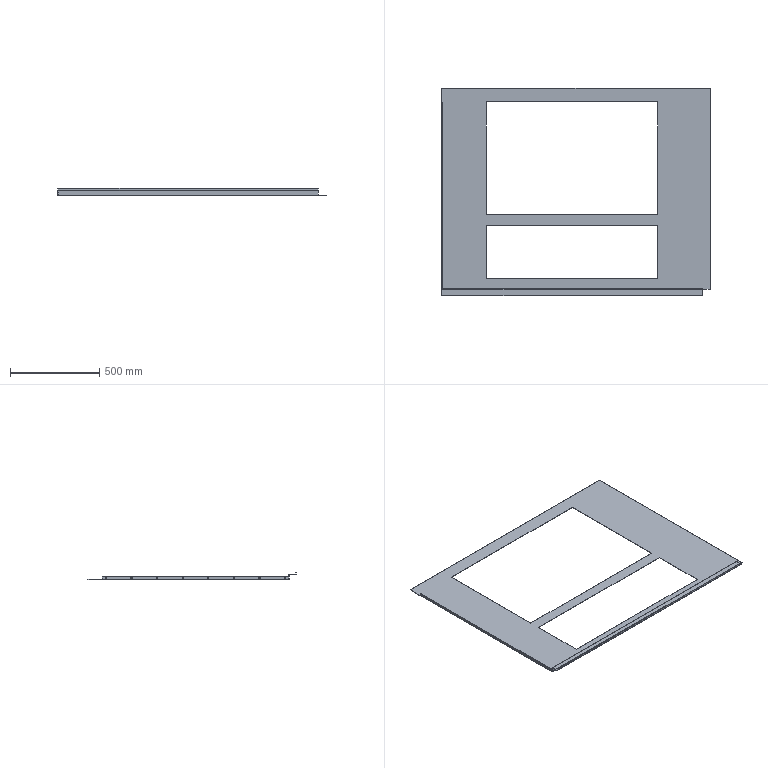Part | STEP file | Rear Plate | 1 solid | 58 faces | box 1504 x 1166 x 40 mm | volume 1850918 mm3 | plane 31 | cylinder 27 | commonest cylinder face diameters 7 x16 1 x7 5 x4